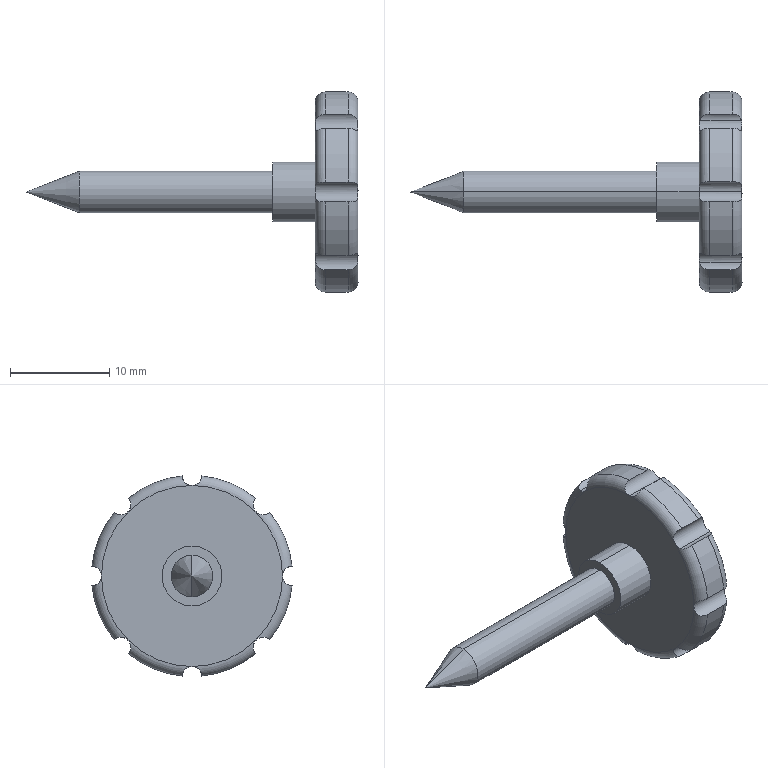Part | SolidWorks | features SavedExtBody 1 | 1 solid | 44 faces | box 33.456 x 20.157 x 20.157 mm | volume 1733 mm3 | cylinder 23 | torus 16 | plane 3 | cone 2 | commonest cylinder face diameters 2 x11 20.256 x8 4.217 x2 6.043 x2